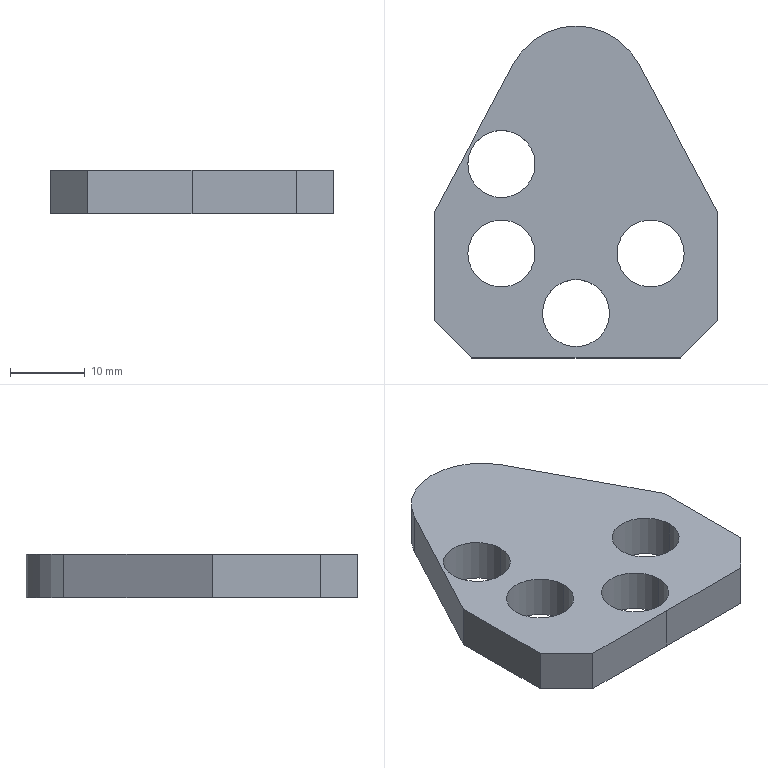Part | CATIA | 1 solid | 20 faces | box 38 x 44.5 x 5.8 mm | volume 6197 mm3 | plane 10 | cylinder 10 | commonest cylinder face diameters 9 x8 19 x2
STEP:
#1=CARTESIAN_POINT('',(19.,-15.498,-5.8));
#2=VERTEX_POINT('',#1);
#3=CARTESIAN_POINT('',(8.388,4.46,-5.8));
#4=VERTEX_POINT('',#3);
#5=CARTESIAN_POINT('',(13.694,-5.519,-5.8));
#6=DIRECTION('',(-0.4695,0.8829,0.));
#7=VECTOR('',#6,1.);
#8=LINE('',#5,#7);
#9=EDGE_CURVE('',#2,#4,#8,.T.);
#10=ORIENTED_EDGE('',*,*,#9,.T.);
#11=CARTESIAN_POINT('',(8.388,4.46,0.));
#12=VERTEX_POINT('',#11);
#13=CARTESIAN_POINT('',(8.388,4.46,-2.9));
#14=DIRECTION('',(0.,0.,-1.));
#15=VECTOR('',#14,1.);
#16=LINE('',#13,#15);
#17=EDGE_CURVE('',#12,#4,#16,.T.);
#18=ORIENTED_EDGE('',*,*,#17,.F.);
#19=CARTESIAN_POINT('',(19.,-15.498,0.));
#20=VERTEX_POINT('',#19);
#21=CARTESIAN_POINT('',(13.694,-5.519,0.));
#22=DIRECTION('',(-0.4695,0.8829,0.));
#23=VECTOR('',#22,1.);
#24=LINE('',#21,#23);
#25=EDGE_CURVE('',#20,#12,#24,.T.);
#26=ORIENTED_EDGE('',*,*,#25,.F.);
#27=CARTESIAN_POINT('',(19.,-15.498,-2.9));
#28=DIRECTION('',(0.,0.,-1.));
#29=VECTOR('',#28,1.);
#30=LINE('',#27,#29);
#31=EDGE_CURVE('',#20,#2,#30,.T.);
#32=ORIENTED_EDGE('',*,*,#31,.T.);
#33=EDGE_LOOP('',(#10,#18,#26,#32));
#34=FACE_OUTER_BOUND('',#33,.T.);
#35=CARTESIAN_POINT('',(19.,-15.498,0.));
#36=DIRECTION('',(-0.8829,-0.4695,0.));
#37=DIRECTION('',(-0.4695,0.8829,0.));
#38=AXIS2_PLACEMENT_3D('',#35,#36,#37);
#39=PLANE('',#38);
#40=ADVANCED_FACE('',(#34),#39,.F.);
#41=CARTESIAN_POINT('',(0.,9.5,-5.8));
#42=VERTEX_POINT('',#41);
#43=CARTESIAN_POINT('',(0.,0.,-5.8));
#44=DIRECTION('',(0.,0.,1.));
#45=AXIS2_PLACEMENT_3D('',#43,#44,$);
#46=CIRCLE('',#45,9.5);
#47=EDGE_CURVE('',#4,#42,#46,.T.);
#48=ORIENTED_EDGE('',*,*,#47,.T.);
#49=CARTESIAN_POINT('',(0.,9.5,0.));
#50=VERTEX_POINT('',#49);
#51=CARTESIAN_POINT('',(0.,9.5,-2.9));
#52=DIRECTION('',(0.,0.,1.));
#53=VECTOR('',#52,1.);
#54=LINE('',#51,#53);
#55=EDGE_CURVE('',#50,#42,#54,.F.);
#56=ORIENTED_EDGE('',*,*,#55,.F.);
#57=CARTESIAN_POINT('',(0.,0.,0.));
#58=DIRECTION('',(0.,0.,1.));
#59=AXIS2_PLACEMENT_3D('',#57,#58,$);
#60=CIRCLE('',#59,9.5);
#61=EDGE_CURVE('',#12,#50,#60,.T.);
#62=ORIENTED_EDGE('',*,*,#61,.F.);
#63=ORIENTED_EDGE('',*,*,#17,.T.);
#64=EDGE_LOOP('',(#48,#56,#62,#63));
#65=FACE_OUTER_BOUND('',#64,.T.);
#66=CARTESIAN_POINT('',(0.,0.,-2.9));
#67=DIRECTION('',(0.,0.,1.));
#68=DIRECTION('',(0.8829,0.4695,0.));
#69=AXIS2_PLACEMENT_3D('',#66,#67,#68);
#70=CYLINDRICAL_SURFACE('',#69,9.5);
#71=ADVANCED_FACE('',(#65),#70,.T.);
#72=CARTESIAN_POINT('',(-8.388,4.46,-5.8));
#73=VERTEX_POINT('',#72);
#74=CARTESIAN_POINT('',(0.,0.,-5.8));
#75=DIRECTION('',(0.,0.,1.));
#76=AXIS2_PLACEMENT_3D('',#74,#75,$);
#77=CIRCLE('',#76,9.5);
#78=EDGE_CURVE('',#42,#73,#77,.T.);
#79=ORIENTED_EDGE('',*,*,#78,.T.);
#80=CARTESIAN_POINT('',(-8.388,4.46,0.));
#81=VERTEX_POINT('',#80);
#82=CARTESIAN_POINT('',(-8.388,4.46,-2.9));
#83=DIRECTION('',(0.,0.,1.));
#84=VECTOR('',#83,1.);
#85=LINE('',#82,#84);
#86=EDGE_CURVE('',#81,#73,#85,.F.);
#87=ORIENTED_EDGE('',*,*,#86,.F.);
#88=CARTESIAN_POINT('',(0.,0.,0.));
#89=DIRECTION('',(0.,0.,1.));
#90=AXIS2_PLACEMENT_3D('',#88,#89,$);
#91=CIRCLE('',#90,9.5);
#92=EDGE_CURVE('',#50,#81,#91,.T.);
#93=ORIENTED_EDGE('',*,*,#92,.F.);
#94=ORIENTED_EDGE('',*,*,#55,.T.);
#95=EDGE_LOOP('',(#79,#87,#93,#94));
#96=FACE_OUTER_BOUND('',#95,.T.);
#97=ADVANCED_FACE('',(#96),#70,.T.);
#98=CARTESIAN_POINT('',(-19.,-15.498,-5.8));
#99=VERTEX_POINT('',#98);
#100=CARTESIAN_POINT('',(-13.694,-5.519,-5.8));
#101=DIRECTION('',(-0.4695,-0.8829,0.));
#102=VECTOR('',#101,1.);
#103=LINE('',#100,#102);
#104=EDGE_CURVE('',#73,#99,#103,.T.);
#105=ORIENTED_EDGE('',*,*,#104,.T.);
#106=CARTESIAN_POINT('',(-19.,-15.498,0.));
#107=VERTEX_POINT('',#106);
#108=CARTESIAN_POINT('',(-19.,-15.498,-2.9));
#109=DIRECTION('',(0.,0.,-1.));
#110=VECTOR('',#109,1.);
#111=LINE('',#108,#110);
#112=EDGE_CURVE('',#107,#99,#111,.T.);
#113=ORIENTED_EDGE('',*,*,#112,.F.);
#114=CARTESIAN_POINT('',(-13.694,-5.519,0.));
#115=DIRECTION('',(-0.4695,-0.8829,0.));
#116=VECTOR('',#115,1.);
#117=LINE('',#114,#116);
#118=EDGE_CURVE('',#81,#107,#117,.T.);
#119=ORIENTED_EDGE('',*,*,#118,.F.);
#120=ORIENTED_EDGE('',*,*,#86,.T.);
#121=EDGE_LOOP('',(#105,#113,#119,#120));
#122=FACE_OUTER_BOUND('',#121,.T.);
#123=CARTESIAN_POINT('',(-8.388,4.46,0.));
#124=DIRECTION('',(0.8829,-0.4695,0.));
#125=DIRECTION('',(-0.4695,-0.8829,0.));
#126=AXIS2_PLACEMENT_3D('',#123,#124,#125);
#127=PLANE('',#126);
#128=ADVANCED_FACE('',(#122),#127,.F.);
#129=CARTESIAN_POINT('',(-19.,-30.,-5.8));
#130=VERTEX_POINT('',#129);
#131=CARTESIAN_POINT('',(-19.,-22.749,-5.8));
#132=DIRECTION('',(0.,-1.,0.));
#133=VECTOR('',#132,1.);
#134=LINE('',#131,#133);
#135=EDGE_CURVE('',#99,#130,#134,.T.);
#136=ORIENTED_EDGE('',*,*,#135,.T.);
#137=CARTESIAN_POINT('',(-19.,-30.,0.));
#138=VERTEX_POINT('',#137);
#139=CARTESIAN_POINT('',(-19.,-30.,-2.9));
#140=DIRECTION('',(0.,0.,-1.));
#141=VECTOR('',#140,1.);
#142=LINE('',#139,#141);
#143=EDGE_CURVE('',#138,#130,#142,.T.);
#144=ORIENTED_EDGE('',*,*,#143,.F.);
#145=CARTESIAN_POINT('',(-19.,-22.749,0.));
#146=DIRECTION('',(0.,-1.,0.));
#147=VECTOR('',#146,1.);
#148=LINE('',#145,#147);
#149=EDGE_CURVE('',#107,#138,#148,.T.);
#150=ORIENTED_EDGE('',*,*,#149,.F.);
#151=ORIENTED_EDGE('',*,*,#112,.T.);
#152=EDGE_LOOP('',(#136,#144,#150,#151));
#153=FACE_OUTER_BOUND('',#152,.T.);
#154=CARTESIAN_POINT('',(-19.,-15.498,0.));
#155=DIRECTION('',(1.,0.,0.));
#156=DIRECTION('',(0.,-1.,0.));
#157=AXIS2_PLACEMENT_3D('',#154,#155,#156);
#158=PLANE('',#157);
#159=ADVANCED_FACE('',(#153),#158,.F.);
#160=CARTESIAN_POINT('',(-14.,-35.,-5.8));
#161=VERTEX_POINT('',#160);
#162=CARTESIAN_POINT('',(-16.5,-32.5,-5.8));
#163=DIRECTION('',(0.7071,-0.7071,0.));
#164=VECTOR('',#163,1.);
#165=LINE('',#162,#164);
#166=EDGE_CURVE('',#130,#161,#165,.T.);
#167=ORIENTED_EDGE('',*,*,#166,.T.);
#168=CARTESIAN_POINT('',(-14.,-35.,0.));
#169=VERTEX_POINT('',#168);
#170=CARTESIAN_POINT('',(-14.,-35.,-2.9));
#171=DIRECTION('',(0.,0.,-1.));
#172=VECTOR('',#171,1.);
#173=LINE('',#170,#172);
#174=EDGE_CURVE('',#169,#161,#173,.T.);
#175=ORIENTED_EDGE('',*,*,#174,.F.);
#176=CARTESIAN_POINT('',(-16.5,-32.5,0.));
#177=DIRECTION('',(0.7071,-0.7071,0.));
#178=VECTOR('',#177,1.);
#179=LINE('',#176,#178);
#180=EDGE_CURVE('',#138,#169,#179,.T.);
#181=ORIENTED_EDGE('',*,*,#180,.F.);
#182=ORIENTED_EDGE('',*,*,#143,.T.);
#183=EDGE_LOOP('',(#167,#175,#181,#182));
#184=FACE_OUTER_BOUND('',#183,.T.);
#185=CARTESIAN_POINT('',(-19.,-30.,0.));
#186=DIRECTION('',(0.7071,0.7071,0.));
#187=DIRECTION('',(0.7071,-0.7071,0.));
#188=AXIS2_PLACEMENT_3D('',#185,#186,#187);
#189=PLANE('',#188);
#190=ADVANCED_FACE('',(#184),#189,.F.);
#191=CARTESIAN_POINT('',(0.,-35.,-5.8));
#192=VERTEX_POINT('',#191);
#193=CARTESIAN_POINT('',(-7.,-35.,-5.8));
#194=DIRECTION('',(1.,0.,0.));
#195=VECTOR('',#194,1.);
#196=LINE('',#193,#195);
#197=EDGE_CURVE('',#161,#192,#196,.T.);
#198=ORIENTED_EDGE('',*,*,#197,.T.);
#199=CARTESIAN_POINT('',(0.,-35.,0.));
#200=VERTEX_POINT('',#199);
#201=CARTESIAN_POINT('',(0.,-35.,-2.9));
#202=DIRECTION('',(0.,0.,-1.));
#203=VECTOR('',#202,1.);
#204=LINE('',#201,#203);
#205=EDGE_CURVE('',#200,#192,#204,.T.);
#206=ORIENTED_EDGE('',*,*,#205,.F.);
#207=CARTESIAN_POINT('',(-7.,-35.,0.));
#208=DIRECTION('',(1.,0.,0.));
#209=VECTOR('',#208,1.);
#210=LINE('',#207,#209);
#211=EDGE_CURVE('',#169,#200,#210,.T.);
#212=ORIENTED_EDGE('',*,*,#211,.F.);
#213=ORIENTED_EDGE('',*,*,#174,.T.);
#214=EDGE_LOOP('',(#198,#206,#212,#213));
#215=FACE_OUTER_BOUND('',#214,.T.);
#216=CARTESIAN_POINT('',(-14.,-35.,0.));
#217=DIRECTION('',(0.,1.,0.));
#218=DIRECTION('',(1.,0.,0.));
#219=AXIS2_PLACEMENT_3D('',#216,#217,#218);
#220=PLANE('',#219);
#221=ADVANCED_FACE('',(#215),#220,.F.);
#222=CARTESIAN_POINT('',(14.,-35.,-5.8));
#223=VERTEX_POINT('',#222);
#224=CARTESIAN_POINT('',(7.,-35.,-5.8));
#225=DIRECTION('',(1.,0.,0.));
#226=VECTOR('',#225,1.);
#227=LINE('',#224,#226);
#228=EDGE_CURVE('',#192,#223,#227,.T.);
#229=ORIENTED_EDGE('',*,*,#228,.T.);
#230=CARTESIAN_POINT('',(14.,-35.,0.));
#231=VERTEX_POINT('',#230);
#232=CARTESIAN_POINT('',(14.,-35.,-2.9));
#233=DIRECTION('',(0.,0.,-1.));
#234=VECTOR('',#233,1.);
#235=LINE('',#232,#234);
#236=EDGE_CURVE('',#231,#223,#235,.T.);
#237=ORIENTED_EDGE('',*,*,#236,.F.);
#238=CARTESIAN_POINT('',(7.,-35.,0.));
#239=DIRECTION('',(1.,0.,0.));
#240=VECTOR('',#239,1.);
#241=LINE('',#238,#240);
#242=EDGE_CURVE('',#200,#231,#241,.T.);
#243=ORIENTED_EDGE('',*,*,#242,.F.);
#244=ORIENTED_EDGE('',*,*,#205,.T.);
#245=EDGE_LOOP('',(#229,#237,#243,#244));
#246=FACE_OUTER_BOUND('',#245,.T.);
#247=ADVANCED_FACE('',(#246),#220,.F.);
#248=CARTESIAN_POINT('',(19.,-30.,-5.8));
#249=VERTEX_POINT('',#248);
#250=CARTESIAN_POINT('',(16.5,-32.5,-5.8));
#251=DIRECTION('',(0.7071,0.7071,0.));
#252=VECTOR('',#251,1.);
#253=LINE('',#250,#252);
#254=EDGE_CURVE('',#223,#249,#253,.T.);
#255=ORIENTED_EDGE('',*,*,#254,.T.);
#256=CARTESIAN_POINT('',(19.,-30.,0.));
#257=VERTEX_POINT('',#256);
#258=CARTESIAN_POINT('',(19.,-30.,-2.9));
#259=DIRECTION('',(0.,0.,-1.));
#260=VECTOR('',#259,1.);
#261=LINE('',#258,#260);
#262=EDGE_CURVE('',#257,#249,#261,.T.);
#263=ORIENTED_EDGE('',*,*,#262,.F.);
#264=CARTESIAN_POINT('',(16.5,-32.5,0.));
#265=DIRECTION('',(0.7071,0.7071,0.));
#266=VECTOR('',#265,1.);
#267=LINE('',#264,#266);
#268=EDGE_CURVE('',#231,#257,#267,.T.);
#269=ORIENTED_EDGE('',*,*,#268,.F.);
#270=ORIENTED_EDGE('',*,*,#236,.T.);
#271=EDGE_LOOP('',(#255,#263,#269,#270));
#272=FACE_OUTER_BOUND('',#271,.T.);
#273=CARTESIAN_POINT('',(14.,-35.,0.));
#274=DIRECTION('',(-0.7071,0.7071,0.));
#275=DIRECTION('',(0.7071,0.7071,0.));
#276=AXIS2_PLACEMENT_3D('',#273,#274,#275);
#277=PLANE('',#276);
#278=ADVANCED_FACE('',(#272),#277,.F.);
#279=CARTESIAN_POINT('',(19.,-22.749,-5.8));
#280=DIRECTION('',(0.,1.,0.));
#281=VECTOR('',#280,1.);
#282=LINE('',#279,#281);
#283=EDGE_CURVE('',#249,#2,#282,.T.);
#284=ORIENTED_EDGE('',*,*,#283,.T.);
#285=ORIENTED_EDGE('',*,*,#31,.F.);
#286=CARTESIAN_POINT('',(19.,-22.749,0.));
#287=DIRECTION('',(0.,1.,0.));
#288=VECTOR('',#287,1.);
#289=LINE('',#286,#288);
#290=EDGE_CURVE('',#257,#20,#289,.T.);
#291=ORIENTED_EDGE('',*,*,#290,.F.);
#292=ORIENTED_EDGE('',*,*,#262,.T.);
#293=EDGE_LOOP('',(#284,#285,#291,#292));
#294=FACE_OUTER_BOUND('',#293,.T.);
#295=CARTESIAN_POINT('',(19.,-30.,0.));
#296=DIRECTION('',(-1.,0.,0.));
#297=DIRECTION('',(0.,1.,0.));
#298=AXIS2_PLACEMENT_3D('',#295,#296,#297);
#299=PLANE('',#298);
#300=ADVANCED_FACE('',(#294),#299,.F.);
#301=CARTESIAN_POINT('',(-4.5,-29.,0.));
#302=VERTEX_POINT('',#301);
#303=CARTESIAN_POINT('',(-4.5,-29.,-5.8));
#304=VERTEX_POINT('',#303);
#305=CARTESIAN_POINT('',(-4.5,-29.,-2.9));
#306=DIRECTION('',(0.,0.,1.));
#307=VECTOR('',#306,1.);
#308=LINE('',#305,#307);
#309=EDGE_CURVE('',#302,#304,#308,.F.);
#310=ORIENTED_EDGE('',*,*,#309,.F.);
#311=CARTESIAN_POINT('',(4.5,-29.,0.));
#312=VERTEX_POINT('',#311);
#313=CARTESIAN_POINT('',(0.,-29.,0.));
#314=DIRECTION('',(0.,0.,1.));
#315=AXIS2_PLACEMENT_3D('',#313,#314,$);
#316=CIRCLE('',#315,4.5);
#317=EDGE_CURVE('',#302,#312,#316,.T.);
#318=ORIENTED_EDGE('',*,*,#317,.T.);
#319=CARTESIAN_POINT('',(4.5,-29.,-5.8));
#320=VERTEX_POINT('',#319);
#321=CARTESIAN_POINT('',(4.5,-29.,-2.9));
#322=DIRECTION('',(0.,0.,1.));
#323=VECTOR('',#322,1.);
#324=LINE('',#321,#323);
#325=EDGE_CURVE('',#312,#320,#324,.F.);
#326=ORIENTED_EDGE('',*,*,#325,.T.);
#327=CARTESIAN_POINT('',(0.,-29.,-5.8));
#328=DIRECTION('',(0.,0.,1.));
#329=AXIS2_PLACEMENT_3D('',#327,#328,$);
#330=CIRCLE('',#329,4.5);
#331=EDGE_CURVE('',#304,#320,#330,.T.);
#332=ORIENTED_EDGE('',*,*,#331,.F.);
#333=EDGE_LOOP('',(#310,#318,#326,#332));
#334=FACE_OUTER_BOUND('',#333,.T.);
#335=CARTESIAN_POINT('',(0.,-29.,-2.9));
#336=DIRECTION('',(0.,0.,1.));
#337=DIRECTION('',(1.,0.,0.));
#338=AXIS2_PLACEMENT_3D('',#335,#336,#337);
#339=CYLINDRICAL_SURFACE('',#338,4.5);
#340=ADVANCED_FACE('',(#334),#339,.F.);
#341=ORIENTED_EDGE('',*,*,#325,.F.);
#342=CARTESIAN_POINT('',(0.,-29.,0.));
#343=DIRECTION('',(0.,0.,1.));
#344=AXIS2_PLACEMENT_3D('',#342,#343,$);
#345=CIRCLE('',#344,4.5);
#346=EDGE_CURVE('',#312,#302,#345,.T.);
#347=ORIENTED_EDGE('',*,*,#346,.T.);
#348=ORIENTED_EDGE('',*,*,#309,.T.);
#349=CARTESIAN_POINT('',(0.,-29.,-5.8));
#350=DIRECTION('',(0.,0.,1.));
#351=AXIS2_PLACEMENT_3D('',#349,#350,$);
#352=CIRCLE('',#351,4.5);
#353=EDGE_CURVE('',#320,#304,#352,.T.);
#354=ORIENTED_EDGE('',*,*,#353,.F.);
#355=EDGE_LOOP('',(#341,#347,#348,#354));
#356=FACE_OUTER_BOUND('',#355,.T.);
#357=ADVANCED_FACE('',(#356),#339,.F.);
#358=CARTESIAN_POINT('',(-14.5,-9.,0.));
#359=VERTEX_POINT('',#358);
#360=CARTESIAN_POINT('',(-14.5,-9.,-5.8));
#361=VERTEX_POINT('',#360);
#362=CARTESIAN_POINT('',(-14.5,-9.,-2.9));
#363=DIRECTION('',(0.,0.,1.));
#364=VECTOR('',#363,1.);
#365=LINE('',#362,#364);
#366=EDGE_CURVE('',#359,#361,#365,.F.);
#367=ORIENTED_EDGE('',*,*,#366,.F.);
#368=CARTESIAN_POINT('',(-5.5,-9.,0.));
#369=VERTEX_POINT('',#368);
#370=CARTESIAN_POINT('',(-10.,-9.,0.));
#371=DIRECTION('',(0.,0.,1.));
#372=AXIS2_PLACEMENT_3D('',#370,#371,$);
#373=CIRCLE('',#372,4.5);
#374=EDGE_CURVE('',#359,#369,#373,.T.);
#375=ORIENTED_EDGE('',*,*,#374,.T.);
#376=CARTESIAN_POINT('',(-5.5,-9.,-5.8));
#377=VERTEX_POINT('',#376);
#378=CARTESIAN_POINT('',(-5.5,-9.,-2.9));
#379=DIRECTION('',(0.,0.,1.));
#380=VECTOR('',#379,1.);
#381=LINE('',#378,#380);
#382=EDGE_CURVE('',#369,#377,#381,.F.);
#383=ORIENTED_EDGE('',*,*,#382,.T.);
#384=CARTESIAN_POINT('',(-10.,-9.,-5.8));
#385=DIRECTION('',(0.,0.,1.));
#386=AXIS2_PLACEMENT_3D('',#384,#385,$);
#387=CIRCLE('',#386,4.5);
#388=EDGE_CURVE('',#361,#377,#387,.T.);
#389=ORIENTED_EDGE('',*,*,#388,.F.);
#390=EDGE_LOOP('',(#367,#375,#383,#389));
#391=FACE_OUTER_BOUND('',#390,.T.);
#392=CARTESIAN_POINT('',(-10.,-9.,-2.9));
#393=DIRECTION('',(0.,0.,1.));
#394=DIRECTION('',(1.,0.,0.));
#395=AXIS2_PLACEMENT_3D('',#392,#393,#394);
#396=CYLINDRICAL_SURFACE('',#395,4.5);
#397=ADVANCED_FACE('',(#391),#396,.F.);
#398=ORIENTED_EDGE('',*,*,#382,.F.);
#399=CARTESIAN_POINT('',(-10.,-9.,0.));
#400=DIRECTION('',(0.,0.,1.));
#401=AXIS2_PLACEMENT_3D('',#399,#400,$);
#402=CIRCLE('',#401,4.5);
#403=EDGE_CURVE('',#369,#359,#402,.T.);
#404=ORIENTED_EDGE('',*,*,#403,.T.);
#405=ORIENTED_EDGE('',*,*,#366,.T.);
#406=CARTESIAN_POINT('',(-10.,-9.,-5.8));
#407=DIRECTION('',(0.,0.,1.));
#408=AXIS2_PLACEMENT_3D('',#406,#407,$);
#409=CIRCLE('',#408,4.5);
#410=EDGE_CURVE('',#377,#361,#409,.T.);
#411=ORIENTED_EDGE('',*,*,#410,.F.);
#412=EDGE_LOOP('',(#398,#404,#405,#411));
#413=FACE_OUTER_BOUND('',#412,.T.);
#414=ADVANCED_FACE('',(#413),#396,.F.);
#415=CARTESIAN_POINT('',(-14.5,-21.,0.));
#416=VERTEX_POINT('',#415);
#417=CARTESIAN_POINT('',(-14.5,-21.,-5.8));
#418=VERTEX_POINT('',#417);
#419=CARTESIAN_POINT('',(-14.5,-21.,-2.9));
#420=DIRECTION('',(0.,0.,1.));
#421=VECTOR('',#420,1.);
#422=LINE('',#419,#421);
#423=EDGE_CURVE('',#416,#418,#422,.F.);
#424=ORIENTED_EDGE('',*,*,#423,.F.);
#425=CARTESIAN_POINT('',(-5.5,-21.,0.));
#426=VERTEX_POINT('',#425);
#427=CARTESIAN_POINT('',(-10.,-21.,0.));
#428=DIRECTION('',(0.,0.,1.));
#429=AXIS2_PLACEMENT_3D('',#427,#428,$);
#430=CIRCLE('',#429,4.5);
#431=EDGE_CURVE('',#416,#426,#430,.T.);
#432=ORIENTED_EDGE('',*,*,#431,.T.);
#433=CARTESIAN_POINT('',(-5.5,-21.,-5.8));
#434=VERTEX_POINT('',#433);
#435=CARTESIAN_POINT('',(-5.5,-21.,-2.9));
#436=DIRECTION('',(0.,0.,1.));
#437=VECTOR('',#436,1.);
#438=LINE('',#435,#437);
#439=EDGE_CURVE('',#426,#434,#438,.F.);
#440=ORIENTED_EDGE('',*,*,#439,.T.);
#441=CARTESIAN_POINT('',(-10.,-21.,-5.8));
#442=DIRECTION('',(0.,0.,1.));
#443=AXIS2_PLACEMENT_3D('',#441,#442,$);
#444=CIRCLE('',#443,4.5);
#445=EDGE_CURVE('',#418,#434,#444,.T.);
#446=ORIENTED_EDGE('',*,*,#445,.F.);
#447=EDGE_LOOP('',(#424,#432,#440,#446));
#448=FACE_OUTER_BOUND('',#447,.T.);
#449=CARTESIAN_POINT('',(-10.,-21.,-2.9));
#450=DIRECTION('',(0.,0.,1.));
#451=DIRECTION('',(1.,0.,0.));
#452=AXIS2_PLACEMENT_3D('',#449,#450,#451);
#453=CYLINDRICAL_SURFACE('',#452,4.5);
#454=ADVANCED_FACE('',(#448),#453,.F.);
#455=ORIENTED_EDGE('',*,*,#439,.F.);
#456=CARTESIAN_POINT('',(-10.,-21.,0.));
#457=DIRECTION('',(0.,0.,1.));
#458=AXIS2_PLACEMENT_3D('',#456,#457,$);
#459=CIRCLE('',#458,4.5);
#460=EDGE_CURVE('',#426,#416,#459,.T.);
#461=ORIENTED_EDGE('',*,*,#460,.T.);
#462=ORIENTED_EDGE('',*,*,#423,.T.);
#463=CARTESIAN_POINT('',(-10.,-21.,-5.8));
#464=DIRECTION('',(0.,0.,1.));
#465=AXIS2_PLACEMENT_3D('',#463,#464,$);
#466=CIRCLE('',#465,4.5);
#467=EDGE_CURVE('',#434,#418,#466,.T.);
#468=ORIENTED_EDGE('',*,*,#467,.F.);
#469=EDGE_LOOP('',(#455,#461,#462,#468));
#470=FACE_OUTER_BOUND('',#469,.T.);
#471=ADVANCED_FACE('',(#470),#453,.F.);
#472=CARTESIAN_POINT('',(5.5,-21.,0.));
#473=VERTEX_POINT('',#472);
#474=CARTESIAN_POINT('',(5.5,-21.,-5.8));
#475=VERTEX_POINT('',#474);
#476=CARTESIAN_POINT('',(5.5,-21.,-2.9));
#477=DIRECTION('',(0.,0.,1.));
#478=VECTOR('',#477,1.);
#479=LINE('',#476,#478);
#480=EDGE_CURVE('',#473,#475,#479,.F.);
#481=ORIENTED_EDGE('',*,*,#480,.F.);
#482=CARTESIAN_POINT('',(14.5,-21.,0.));
#483=VERTEX_POINT('',#482);
#484=CARTESIAN_POINT('',(10.,-21.,0.));
#485=DIRECTION('',(0.,0.,1.));
#486=AXIS2_PLACEMENT_3D('',#484,#485,$);
#487=CIRCLE('',#486,4.5);
#488=EDGE_CURVE('',#473,#483,#487,.T.);
#489=ORIENTED_EDGE('',*,*,#488,.T.);
#490=CARTESIAN_POINT('',(14.5,-21.,-5.8));
#491=VERTEX_POINT('',#490);
#492=CARTESIAN_POINT('',(14.5,-21.,-2.9));
#493=DIRECTION('',(0.,0.,1.));
#494=VECTOR('',#493,1.);
#495=LINE('',#492,#494);
#496=EDGE_CURVE('',#483,#491,#495,.F.);
#497=ORIENTED_EDGE('',*,*,#496,.T.);
#498=CARTESIAN_POINT('',(10.,-21.,-5.8));
#499=DIRECTION('',(0.,0.,1.));
#500=AXIS2_PLACEMENT_3D('',#498,#499,$);
#501=CIRCLE('',#500,4.5);
#502=EDGE_CURVE('',#475,#491,#501,.T.);
#503=ORIENTED_EDGE('',*,*,#502,.F.);
#504=EDGE_LOOP('',(#481,#489,#497,#503));
#505=FACE_OUTER_BOUND('',#504,.T.);
#506=CARTESIAN_POINT('',(10.,-21.,-2.9));
#507=DIRECTION('',(0.,0.,1.));
#508=DIRECTION('',(1.,0.,0.));
#509=AXIS2_PLACEMENT_3D('',#506,#507,#508);
#510=CYLINDRICAL_SURFACE('',#509,4.5);
#511=ADVANCED_FACE('',(#505),#510,.F.);
#512=ORIENTED_EDGE('',*,*,#496,.F.);
#513=CARTESIAN_POINT('',(10.,-21.,0.));
#514=DIRECTION('',(0.,0.,1.));
#515=AXIS2_PLACEMENT_3D('',#513,#514,$);
#516=CIRCLE('',#515,4.5);
#517=EDGE_CURVE('',#483,#473,#516,.T.);
#518=ORIENTED_EDGE('',*,*,#517,.T.);
#519=ORIENTED_EDGE('',*,*,#480,.T.);
#520=CARTESIAN_POINT('',(10.,-21.,-5.8));
#521=DIRECTION('',(0.,0.,1.));
#522=AXIS2_PLACEMENT_3D('',#520,#521,$);
#523=CIRCLE('',#522,4.5);
#524=EDGE_CURVE('',#491,#475,#523,.T.);
#525=ORIENTED_EDGE('',*,*,#524,.F.);
#526=EDGE_LOOP('',(#512,#518,#519,#525));
#527=FACE_OUTER_BOUND('',#526,.T.);
#528=ADVANCED_FACE('',(#527),#510,.F.);
#529=ORIENTED_EDGE('',*,*,#25,.T.);
#530=ORIENTED_EDGE('',*,*,#61,.T.);
#531=ORIENTED_EDGE('',*,*,#92,.T.);
#532=ORIENTED_EDGE('',*,*,#118,.T.);
#533=ORIENTED_EDGE('',*,*,#149,.T.);
#534=ORIENTED_EDGE('',*,*,#180,.T.);
#535=ORIENTED_EDGE('',*,*,#211,.T.);
#536=ORIENTED_EDGE('',*,*,#242,.T.);
#537=ORIENTED_EDGE('',*,*,#268,.T.);
#538=ORIENTED_EDGE('',*,*,#290,.T.);
#539=EDGE_LOOP('',(#529,#530,#531,#532,#533,#534,#535,#536,#537,#538));
#540=FACE_OUTER_BOUND('',#539,.T.);
#541=ORIENTED_EDGE('',*,*,#317,.F.);
#542=ORIENTED_EDGE('',*,*,#346,.F.);
#543=EDGE_LOOP('',(#541,#542));
#544=FACE_BOUND('',#543,.T.);
#545=ORIENTED_EDGE('',*,*,#374,.F.);
#546=ORIENTED_EDGE('',*,*,#403,.F.);
#547=EDGE_LOOP('',(#545,#546));
#548=FACE_BOUND('',#547,.T.);
#549=ORIENTED_EDGE('',*,*,#431,.F.);
#550=ORIENTED_EDGE('',*,*,#460,.F.);
#551=EDGE_LOOP('',(#549,#550));
#552=FACE_BOUND('',#551,.T.);
#553=ORIENTED_EDGE('',*,*,#488,.F.);
#554=ORIENTED_EDGE('',*,*,#517,.F.);
#555=EDGE_LOOP('',(#553,#554));
#556=FACE_BOUND('',#555,.T.);
#557=CARTESIAN_POINT('',(0.,0.,0.));
#558=DIRECTION('',(0.,0.,1.));
#559=DIRECTION('',(1.,0.,0.));
#560=AXIS2_PLACEMENT_3D('',#557,#558,#559);
#561=PLANE('',#560);
#562=ADVANCED_FACE('',(#540,#544,#548,#552,#556),#561,.T.);
#563=ORIENTED_EDGE('',*,*,#283,.F.);
#564=ORIENTED_EDGE('',*,*,#254,.F.);
#565=ORIENTED_EDGE('',*,*,#228,.F.);
#566=ORIENTED_EDGE('',*,*,#197,.F.);
#567=ORIENTED_EDGE('',*,*,#166,.F.);
#568=ORIENTED_EDGE('',*,*,#135,.F.);
#569=ORIENTED_EDGE('',*,*,#104,.F.);
#570=ORIENTED_EDGE('',*,*,#78,.F.);
#571=ORIENTED_EDGE('',*,*,#47,.F.);
#572=ORIENTED_EDGE('',*,*,#9,.F.);
#573=EDGE_LOOP('',(#563,#564,#565,#566,#567,#568,#569,#570,#571,#572));
#574=FACE_OUTER_BOUND('',#573,.T.);
#575=ORIENTED_EDGE('',*,*,#353,.T.);
#576=ORIENTED_EDGE('',*,*,#331,.T.);
#577=EDGE_LOOP('',(#575,#576));
#578=FACE_BOUND('',#577,.T.);
#579=ORIENTED_EDGE('',*,*,#410,.T.);
#580=ORIENTED_EDGE('',*,*,#388,.T.);
#581=EDGE_LOOP('',(#579,#580));
#582=FACE_BOUND('',#581,.T.);
#583=ORIENTED_EDGE('',*,*,#467,.T.);
#584=ORIENTED_EDGE('',*,*,#445,.T.);
#585=EDGE_LOOP('',(#583,#584));
#586=FACE_BOUND('',#585,.T.);
#587=ORIENTED_EDGE('',*,*,#524,.T.);
#588=ORIENTED_EDGE('',*,*,#502,.T.);
#589=EDGE_LOOP('',(#587,#588));
#590=FACE_BOUND('',#589,.T.);
#591=CARTESIAN_POINT('',(0.,0.,-5.8));
#592=DIRECTION('',(0.,0.,1.));
#593=DIRECTION('',(1.,0.,0.));
#594=AXIS2_PLACEMENT_3D('',#591,#592,#593);
#595=PLANE('',#594);
#596=ADVANCED_FACE('',(#574,#578,#582,#586,#590),#595,.F.);
#597=CLOSED_SHELL('',(#40,#71,#97,#128,#159,#190,#221,#247,#278,#300,#340,#357,#397,#414,#454,#471,#511,#528,#562,#596));
#598=MANIFOLD_SOLID_BREP('',#597);
#599=(LENGTH_UNIT()NAMED_UNIT(*)SI_UNIT(.MILLI.,.METRE.));
#600=UNCERTAINTY_MEASURE_WITH_UNIT(LENGTH_MEASURE(0.005),#599,'','');
#601=(NAMED_UNIT(*)PLANE_ANGLE_UNIT()SI_UNIT($,.RADIAN.));
#602=(NAMED_UNIT(*)SI_UNIT($,.STERADIAN.)SOLID_ANGLE_UNIT());
#603=(GEOMETRIC_REPRESENTATION_CONTEXT(3)GLOBAL_UNCERTAINTY_ASSIGNED_CONTEXT((#600))GLOBAL_UNIT_ASSIGNED_CONTEXT((#599,#601,#602))REPRESENTATION_CONTEXT('',''));
#604=ADVANCED_BREP_SHAPE_REPRESENTATION('',(#598),#603);